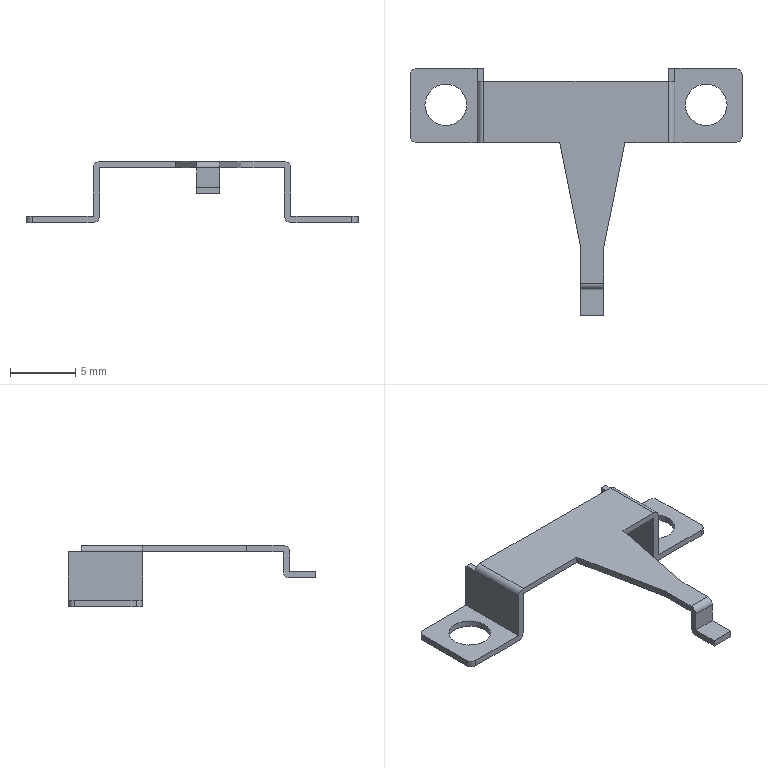Part | STEP file | 0243_106_Sensor_EE-1003A | 1 solid | 42 faces | box 25.5 x 19 x 4.7 mm | volume 99.726 mm3 | plane 28 | cylinder 14 | commonest cylinder face diameters 1 x10 3.2 x4